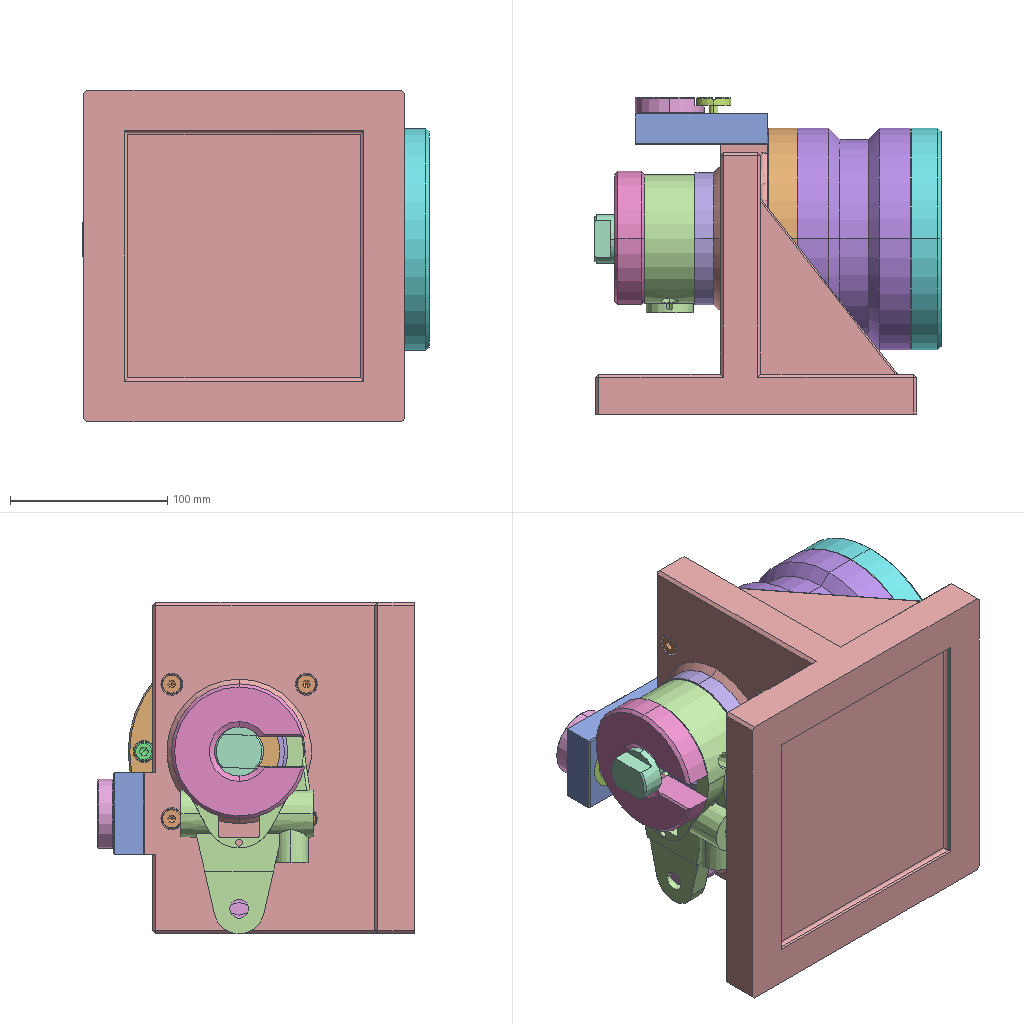Assembly | SolidWorks | 22 different items | 23 placed | box 220 x 202 x 211 mm
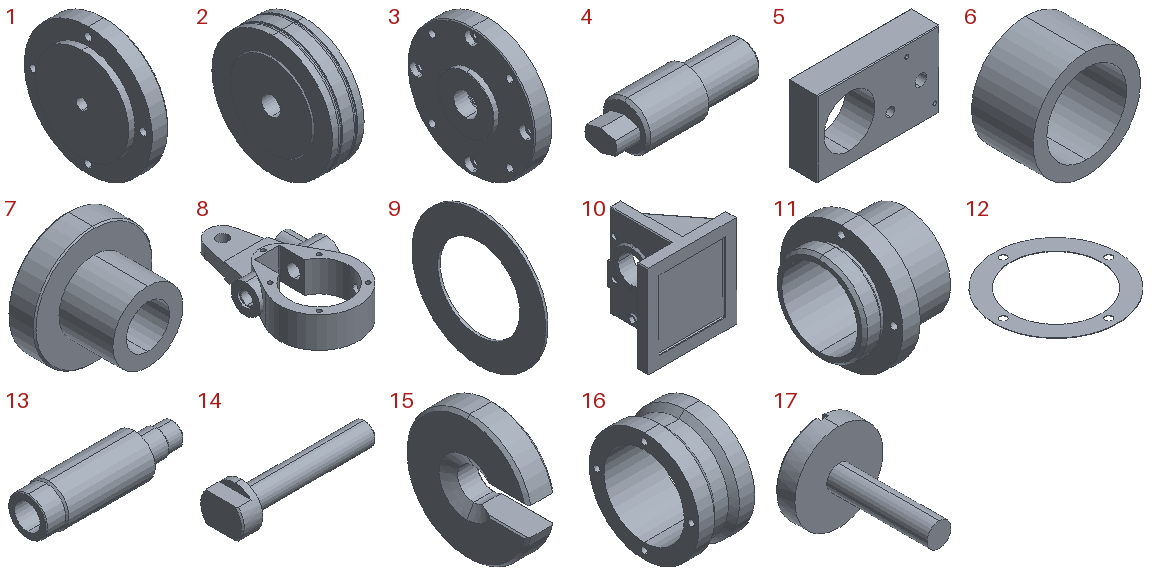Parts list (item | name | quantity | size | volume | features):
1 | - | x1 | 26 x 141 x 141 mm | 338840 mm3 | features ICE 2, Chamfer 1, Revolution 1
2 | - | x1 | 28 x 103.442 x 103.442 mm | 191573 mm3 | features Sweep 2, Chamfer 1, Revolution 1
3 | - | x1 | 32 x 141 x 141 mm | 347487 mm3 | features ICE 3, Chamfer 2, Revolution 2
4 | - | x1 | 54 x 18 x 18 mm | 9866 mm3 | features Chamfer 2, ICE 1, Revolution 1
5 | - | x1 | 84 x 20 x 52 mm | 65474 mm3 | features ICE 5, Chamfer 1, Extrusion 1
6 | - | x1 | 35 x 20 x 35 mm | 8624 mm3 | features Revolution 1
7 | - | x1 | 44 x 30 x 44 mm | 19113 mm3 | features Chamfer 2, ICE 1, Revolution 1
8 | - | x1 | 88 x 157 x 32 mm | 127446 mm3 | features ICE 9, HoleWzd 4, CirPattern 1, Extrusion 1, Fillet 1, RefAxis 1, RevCut 1
9 | - | x1 | 0.5 x 26 x 26 mm | 164.934 mm3 | features Extrusion 1
10 | - | x1 | 204 x 171.5 x 211 mm | 1841584 mm3 | features ICE 19, Fillet 5, Chamfer 3, Extrusion 1
11 | - | x1 | 58.8 x 84 x 84 mm | 80812 mm3 | features Chamfer 2, ICE 2, Revolution 1
12 | - | x2 | 141 x 141 x 0.5 mm | 3541 mm3 | features Extrusion 1, ICE 1
13 | - | x1 | 90.69 x 26 x 26 mm | 34532 mm3 | features Chamfer 3, Revolution 1
14 | - | x1 | 103.85 x 31.18 x 31.18 mm | 28176 mm3 | features Chamfer 2, ICE 1, Revolution 1
15 | - | x1 | 19 x 84.937 x 86 mm | 88865 mm3 | features Chamfer 2, ICE 1, Revolution 1
16 | - | x1 | 71.5 x 141 x 141 mm | 441421 mm3 | features ICE 2, Revolution 1
17 | - | x1 | 22 x 30 x 22 mm | 2536 mm3 | features Chamfer 1, ICE 1, Revolution 1
18 | hex lobular socket head cap screws-4.8 gb | x1 | - | - | -
19 | hex lobular socket thread forming screws gb | x1 | - | - | -
20 | hex nut-fine pitch-style washer-grade ab gb | x1 | - | - | -
21 | parallel pins hardening steel gb | x1 | - | - | -
22 | slotted cheese head screws gb | x1 | - | - | -
Mates (type | each side: item.copy, entity, surface, feature):
Coincident | 10.1 face plane Boss-Extrude1 | 5.1 face plane Boss-Extrude1
Concentric | 10.1 face cylinder Cut-Extrude12 | 5.1 face cylinder Cut-Extrude3
Coincident | 5.1 face plane Boss-Extrude1 | 6.1 face plane Revolve1
Coincident | 5.1 edge | 6.1 edge
Coincident | 6.1 face plane Revolve1 | 7.1 face plane Revolve1
Coincident | 6.1 edge | 7.1 edge
Coincident | 10.1 edge | 3.1 edge
Coincident | 10.1 edge | 11.1 edge
Concentric | 10.1 face cylinder Cut-Extrude11 | 11.1 face cylinder Cut-Extrude1
Coincident | 13.1 face plane Revolve1 | 9.1 face plane Boss-Extrude1
Coincident | 13.1 edge | 9.1 edge
Coincident | 2.1 edge | 9.1 edge
Concentric | 13.1 edge | 14.1 edge
Coincident | 13.1 face plane Revolve1 | 14.1 face plane Revolve1
Concentric | 11.1 face cylinder Revolve1 | 8.1 face cylinder Cut-Extrude1
Coincident | 11.1 face plane Revolve1 | 8.1 face plane Boss-Extrude1
Coincident | 8.1 face plane Boss-Extrude1 | 15.1 face plane Revolve1
Coincident | 8.1 edge | 15.1 edge
Concentric | 14.1 edge | 15.1 edge
Concentric | 14.1 face cone Revolve1 | 15.1 face cone Revolve1
Coincident | 14.1 edge | 15.1 face cone Revolve1
Coincident | 3.1 edge | 12.1 edge
Concentric | 3.1 face cylinder Cut-Extrude2 | 12.1 face cylinder Cut-Extrude1
Coincident | 12.1 edge | 16.1 edge
Concentric | 3.1 face cylinder Cut-Extrude2 | 16.1 face cylinder Cut-Extrude1
Concentric | 16.1 edge | 12.2 edge
Coincident | 16.1 face plane Revolve1 | 12.2 face plane Boss-Extrude1
Coincident | 1.1 edge | 12.2 edge
Concentric | 1.1 face cylinder Cut-Extrude1 | 16.1 face cylinder Cut-Extrude2
Concentric | 5.1 face cylinder Cut-Extrude2 | 17.1 face cylinder Revolve1
Coincident | 7.1 face plane Cut-Extrude1 | 17.1 face plane Revolve1
Concentric | 10.1 face cylinder Cut-Extrude13 | 8.1 face cylinder Ø12.0 (12) Diameter Hole1
Coincident | 10.1 edge | 4.1 edge